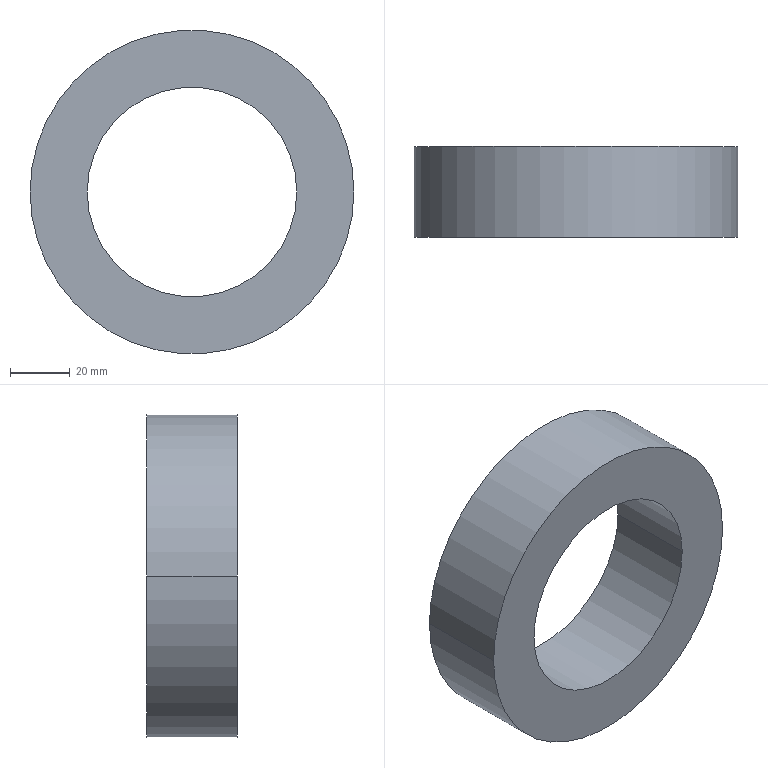Part | STEP file | W468 | 1 solid | 6 faces | box 108.1 x 30.3 x 108.1 mm | volume 161481 mm3 | cylinder 4 | plane 2 | commonest cylinder face diameters 70 x2 108.1 x2
STEP:
#1=CARTESIAN_POINT('',(0.,0.,0.));
#2=DIRECTION('',(0.,0.,1.));
#3=DIRECTION('',(1.,0.,0.));
#4=AXIS2_PLACEMENT_3D('',#1,#2,#3);
#5=CARTESIAN_POINT('',(54.05,0.,0.));
#6=VERTEX_POINT('',#5);
#7=CARTESIAN_POINT('',(-54.05,0.,0.));
#8=VERTEX_POINT('',#7);
#9=CARTESIAN_POINT('',(0.,0.,0.));
#10=DIRECTION('',(0.,-1.,0.));
#11=DIRECTION('',(1.,0.,0.));
#12=AXIS2_PLACEMENT_3D('',#9,#10,#11);
#13=CIRCLE('',#12,54.05);
#14=CARTESIAN_POINT('',(0.,0.,0.));
#15=DIRECTION('',(0.,-1.,0.));
#16=DIRECTION('',(-1.,0.,0.));
#17=AXIS2_PLACEMENT_3D('',#14,#15,#16);
#18=PLANE('',#17);
#19=CARTESIAN_POINT('',(0.,0.));
#20=DIRECTION('',(-1.,0.));
#21=AXIS2_PLACEMENT_2D('',#19,#20);
#22=CIRCLE('',#21,54.05);
#23=(GEOMETRIC_REPRESENTATION_CONTEXT(2)PARAMETRIC_REPRESENTATION_CONTEXT()REPRESENTATION_CONTEXT('',''));
#24=DEFINITIONAL_REPRESENTATION('',(#22),#23);
#25=PCURVE('',#18,#24);
#26=CARTESIAN_POINT('',(0.,31.815,0.));
#27=DIRECTION('',(0.,-1.,0.));
#28=DIRECTION('',(-1.,0.,0.));
#29=AXIS2_PLACEMENT_3D('',#26,#27,#28);
#30=CYLINDRICAL_SURFACE('',#29,54.05);
#31=CARTESIAN_POINT('',(3.142,31.815));
#32=DIRECTION('',(1.,0.));
#33=VECTOR('',#32,1.);
#34=LINE('',#31,#33);
#35=(GEOMETRIC_REPRESENTATION_CONTEXT(2)PARAMETRIC_REPRESENTATION_CONTEXT()REPRESENTATION_CONTEXT('',''));
#36=DEFINITIONAL_REPRESENTATION('',(#34),#35);
#37=PCURVE('',#30,#36);
#38=SURFACE_CURVE('',#13,(#25,#37),.PCURVE_S1.);
#39=EDGE_CURVE('',#6,#8,#38,.T.);
#40=ORIENTED_EDGE('',*,*,#39,.F.);
#41=CARTESIAN_POINT('',(0.,0.,0.));
#42=DIRECTION('',(0.,1.,0.));
#43=DIRECTION('',(1.,0.,0.));
#44=AXIS2_PLACEMENT_3D('',#41,#42,#43);
#45=CIRCLE('',#44,54.05);
#46=CARTESIAN_POINT('',(-54.05,0.));
#47=CARTESIAN_POINT('',(-54.05,93.617));
#48=CARTESIAN_POINT('',(27.025,46.809));
#49=CARTESIAN_POINT('',(108.1,0.));
#50=CARTESIAN_POINT('',(27.025,-46.809));
#51=CARTESIAN_POINT('',(-54.05,-93.617));
#52=CARTESIAN_POINT('',(-54.05,0.));
#53=(BOUNDED_CURVE()B_SPLINE_CURVE(2,(#46,#47,#48,#49,#50,#51,#52),.UNSPECIFIED.,.T.,.F.)B_SPLINE_CURVE_WITH_KNOTS((1,2,2,2,2,1),(-2.094,0.,2.094,4.189,6.283,8.378),.UNSPECIFIED.)CURVE()GEOMETRIC_REPRESENTATION_ITEM()RATIONAL_B_SPLINE_CURVE((1.,0.5,1.,0.5,1.,0.5,1.))REPRESENTATION_ITEM(''));
#54=(GEOMETRIC_REPRESENTATION_CONTEXT(2)PARAMETRIC_REPRESENTATION_CONTEXT()REPRESENTATION_CONTEXT('',''));
#55=DEFINITIONAL_REPRESENTATION('',(#53),#54);
#56=PCURVE('',#18,#55);
#57=CARTESIAN_POINT('',(0.,31.815,0.));
#58=DIRECTION('',(0.,-1.,0.));
#59=DIRECTION('',(-1.,0.,0.));
#60=AXIS2_PLACEMENT_3D('',#57,#58,#59);
#61=CYLINDRICAL_SURFACE('',#60,54.05);
#62=CARTESIAN_POINT('',(3.142,31.815));
#63=DIRECTION('',(-1.,0.));
#64=VECTOR('',#63,1.);
#65=LINE('',#62,#64);
#66=(GEOMETRIC_REPRESENTATION_CONTEXT(2)PARAMETRIC_REPRESENTATION_CONTEXT()REPRESENTATION_CONTEXT('',''));
#67=DEFINITIONAL_REPRESENTATION('',(#65),#66);
#68=PCURVE('',#61,#67);
#69=SURFACE_CURVE('',#45,(#56,#68),.PCURVE_S1.);
#70=EDGE_CURVE('',#6,#8,#69,.T.);
#71=ORIENTED_EDGE('',*,*,#70,.T.);
#72=EDGE_LOOP('',(#40,#71));
#73=FACE_BOUND('',#72,.F.);
#74=CARTESIAN_POINT('',(35.,0.,0.));
#75=VERTEX_POINT('',#74);
#76=CARTESIAN_POINT('',(-35.,0.,0.));
#77=VERTEX_POINT('',#76);
#78=CARTESIAN_POINT('',(0.,0.,0.));
#79=DIRECTION('',(0.,1.,0.));
#80=DIRECTION('',(1.,0.,0.));
#81=AXIS2_PLACEMENT_3D('',#78,#79,#80);
#82=CIRCLE('',#81,35.);
#83=CARTESIAN_POINT('',(-35.,0.));
#84=CARTESIAN_POINT('',(-35.,60.622));
#85=CARTESIAN_POINT('',(17.5,30.311));
#86=CARTESIAN_POINT('',(70.,0.));
#87=CARTESIAN_POINT('',(17.5,-30.311));
#88=CARTESIAN_POINT('',(-35.,-60.622));
#89=CARTESIAN_POINT('',(-35.,0.));
#90=(BOUNDED_CURVE()B_SPLINE_CURVE(2,(#83,#84,#85,#86,#87,#88,#89),.UNSPECIFIED.,.T.,.F.)B_SPLINE_CURVE_WITH_KNOTS((1,2,2,2,2,1),(-2.094,0.,2.094,4.189,6.283,8.378),.UNSPECIFIED.)CURVE()GEOMETRIC_REPRESENTATION_ITEM()RATIONAL_B_SPLINE_CURVE((1.,0.5,1.,0.5,1.,0.5,1.))REPRESENTATION_ITEM(''));
#91=(GEOMETRIC_REPRESENTATION_CONTEXT(2)PARAMETRIC_REPRESENTATION_CONTEXT()REPRESENTATION_CONTEXT('',''));
#92=DEFINITIONAL_REPRESENTATION('',(#90),#91);
#93=PCURVE('',#18,#92);
#94=CARTESIAN_POINT('',(0.,31.815,0.));
#95=DIRECTION('',(0.,-1.,0.));
#96=DIRECTION('',(-1.,0.,0.));
#97=AXIS2_PLACEMENT_3D('',#94,#95,#96);
#98=CYLINDRICAL_SURFACE('',#97,35.);
#99=CARTESIAN_POINT('',(3.142,31.815));
#100=DIRECTION('',(-1.,0.));
#101=VECTOR('',#100,1.);
#102=LINE('',#99,#101);
#103=(GEOMETRIC_REPRESENTATION_CONTEXT(2)PARAMETRIC_REPRESENTATION_CONTEXT()REPRESENTATION_CONTEXT('',''));
#104=DEFINITIONAL_REPRESENTATION('',(#102),#103);
#105=PCURVE('',#98,#104);
#106=SURFACE_CURVE('',#82,(#93,#105),.PCURVE_S1.);
#107=EDGE_CURVE('',#75,#77,#106,.T.);
#108=ORIENTED_EDGE('',*,*,#107,.F.);
#109=CARTESIAN_POINT('',(0.,0.,0.));
#110=DIRECTION('',(0.,-1.,0.));
#111=DIRECTION('',(1.,0.,0.));
#112=AXIS2_PLACEMENT_3D('',#109,#110,#111);
#113=CIRCLE('',#112,35.);
#114=CARTESIAN_POINT('',(0.,0.));
#115=DIRECTION('',(-1.,0.));
#116=AXIS2_PLACEMENT_2D('',#114,#115);
#117=CIRCLE('',#116,35.);
#118=(GEOMETRIC_REPRESENTATION_CONTEXT(2)PARAMETRIC_REPRESENTATION_CONTEXT()REPRESENTATION_CONTEXT('',''));
#119=DEFINITIONAL_REPRESENTATION('',(#117),#118);
#120=PCURVE('',#18,#119);
#121=CARTESIAN_POINT('',(0.,31.815,0.));
#122=DIRECTION('',(0.,-1.,0.));
#123=DIRECTION('',(-1.,0.,0.));
#124=AXIS2_PLACEMENT_3D('',#121,#122,#123);
#125=CYLINDRICAL_SURFACE('',#124,35.);
#126=CARTESIAN_POINT('',(3.142,31.815));
#127=DIRECTION('',(1.,0.));
#128=VECTOR('',#127,1.);
#129=LINE('',#126,#128);
#130=(GEOMETRIC_REPRESENTATION_CONTEXT(2)PARAMETRIC_REPRESENTATION_CONTEXT()REPRESENTATION_CONTEXT('',''));
#131=DEFINITIONAL_REPRESENTATION('',(#129),#130);
#132=PCURVE('',#125,#131);
#133=SURFACE_CURVE('',#113,(#120,#132),.PCURVE_S1.);
#134=EDGE_CURVE('',#75,#77,#133,.T.);
#135=ORIENTED_EDGE('',*,*,#134,.T.);
#136=EDGE_LOOP('',(#108,#135));
#137=FACE_BOUND('',#136,.F.);
#138=ADVANCED_FACE('',(#73,#137),#18,.T.);
#139=CARTESIAN_POINT('',(54.05,30.3,0.));
#140=VERTEX_POINT('',#139);
#141=CARTESIAN_POINT('',(-54.05,30.3,0.));
#142=VERTEX_POINT('',#141);
#143=CARTESIAN_POINT('',(0.,30.3,0.));
#144=DIRECTION('',(0.,-1.,0.));
#145=DIRECTION('',(1.,0.,0.));
#146=AXIS2_PLACEMENT_3D('',#143,#144,#145);
#147=CIRCLE('',#146,54.05);
#148=CARTESIAN_POINT('',(3.142,1.515));
#149=DIRECTION('',(1.,0.));
#150=VECTOR('',#149,1.);
#151=LINE('',#148,#150);
#152=(GEOMETRIC_REPRESENTATION_CONTEXT(2)PARAMETRIC_REPRESENTATION_CONTEXT()REPRESENTATION_CONTEXT('',''));
#153=DEFINITIONAL_REPRESENTATION('',(#151),#152);
#154=PCURVE('',#30,#153);
#155=CARTESIAN_POINT('',(0.,30.3,0.));
#156=DIRECTION('',(0.,-1.,0.));
#157=DIRECTION('',(-1.,0.,0.));
#158=AXIS2_PLACEMENT_3D('',#155,#156,#157);
#159=PLANE('',#158);
#160=CARTESIAN_POINT('',(0.,0.));
#161=DIRECTION('',(-1.,0.));
#162=AXIS2_PLACEMENT_2D('',#160,#161);
#163=CIRCLE('',#162,54.05);
#164=(GEOMETRIC_REPRESENTATION_CONTEXT(2)PARAMETRIC_REPRESENTATION_CONTEXT()REPRESENTATION_CONTEXT('',''));
#165=DEFINITIONAL_REPRESENTATION('',(#163),#164);
#166=PCURVE('',#159,#165);
#167=SURFACE_CURVE('',#147,(#154,#166),.PCURVE_S1.);
#168=EDGE_CURVE('',#140,#142,#167,.T.);
#169=ORIENTED_EDGE('',*,*,#168,.T.);
#170=CARTESIAN_POINT('',(-54.05,0.,0.));
#171=DIRECTION('',(0.,1.,0.));
#172=VECTOR('',#171,1.);
#173=LINE('',#170,#172);
#174=CARTESIAN_POINT('',(6.283,31.815));
#175=DIRECTION('',(0.,-1.));
#176=VECTOR('',#175,1.);
#177=LINE('',#174,#176);
#178=(GEOMETRIC_REPRESENTATION_CONTEXT(2)PARAMETRIC_REPRESENTATION_CONTEXT()REPRESENTATION_CONTEXT('',''));
#179=DEFINITIONAL_REPRESENTATION('',(#177),#178);
#180=PCURVE('',#30,#179);
#181=CARTESIAN_POINT('',(0.,31.815));
#182=DIRECTION('',(0.,-1.));
#183=VECTOR('',#182,1.);
#184=LINE('',#181,#183);
#185=(GEOMETRIC_REPRESENTATION_CONTEXT(2)PARAMETRIC_REPRESENTATION_CONTEXT()REPRESENTATION_CONTEXT('',''));
#186=DEFINITIONAL_REPRESENTATION('',(#184),#185);
#187=PCURVE('',#61,#186);
#188=SURFACE_CURVE('',#173,(#180,#187),.PCURVE_S1.);
#189=EDGE_CURVE('',#8,#142,#188,.T.);
#190=ORIENTED_EDGE('',*,*,#189,.F.);
#191=ORIENTED_EDGE('',*,*,#39,.F.);
#192=CARTESIAN_POINT('',(54.05,0.,0.));
#193=DIRECTION('',(0.,1.,0.));
#194=VECTOR('',#193,1.);
#195=LINE('',#192,#194);
#196=CARTESIAN_POINT('',(3.142,31.815));
#197=DIRECTION('',(0.,-1.));
#198=VECTOR('',#197,1.);
#199=LINE('',#196,#198);
#200=(GEOMETRIC_REPRESENTATION_CONTEXT(2)PARAMETRIC_REPRESENTATION_CONTEXT()REPRESENTATION_CONTEXT('',''));
#201=DEFINITIONAL_REPRESENTATION('',(#199),#200);
#202=PCURVE('',#30,#201);
#203=CARTESIAN_POINT('',(3.142,31.815));
#204=DIRECTION('',(0.,-1.));
#205=VECTOR('',#204,1.);
#206=LINE('',#203,#205);
#207=(GEOMETRIC_REPRESENTATION_CONTEXT(2)PARAMETRIC_REPRESENTATION_CONTEXT()REPRESENTATION_CONTEXT('',''));
#208=DEFINITIONAL_REPRESENTATION('',(#206),#207);
#209=PCURVE('',#61,#208);
#210=SURFACE_CURVE('',#195,(#202,#209),.PCURVE_S1.);
#211=EDGE_CURVE('',#6,#140,#210,.T.);
#212=ORIENTED_EDGE('',*,*,#211,.T.);
#213=EDGE_LOOP('',(#169,#190,#191,#212));
#214=FACE_BOUND('',#213,.T.);
#215=ADVANCED_FACE('',(#214),#30,.T.);
#216=ORIENTED_EDGE('',*,*,#70,.T.);
#217=ORIENTED_EDGE('',*,*,#189,.T.);
#218=CARTESIAN_POINT('',(0.,30.3,0.));
#219=DIRECTION('',(0.,1.,0.));
#220=DIRECTION('',(1.,0.,0.));
#221=AXIS2_PLACEMENT_3D('',#218,#219,#220);
#222=CIRCLE('',#221,54.05);
#223=CARTESIAN_POINT('',(3.142,1.515));
#224=DIRECTION('',(-1.,0.));
#225=VECTOR('',#224,1.);
#226=LINE('',#223,#225);
#227=(GEOMETRIC_REPRESENTATION_CONTEXT(2)PARAMETRIC_REPRESENTATION_CONTEXT()REPRESENTATION_CONTEXT('',''));
#228=DEFINITIONAL_REPRESENTATION('',(#226),#227);
#229=PCURVE('',#61,#228);
#230=CARTESIAN_POINT('',(-54.05,0.));
#231=CARTESIAN_POINT('',(-54.05,93.617));
#232=CARTESIAN_POINT('',(27.025,46.809));
#233=CARTESIAN_POINT('',(108.1,0.));
#234=CARTESIAN_POINT('',(27.025,-46.809));
#235=CARTESIAN_POINT('',(-54.05,-93.617));
#236=CARTESIAN_POINT('',(-54.05,0.));
#237=(BOUNDED_CURVE()B_SPLINE_CURVE(2,(#230,#231,#232,#233,#234,#235,#236),.UNSPECIFIED.,.T.,.F.)B_SPLINE_CURVE_WITH_KNOTS((1,2,2,2,2,1),(-2.094,0.,2.094,4.189,6.283,8.378),.UNSPECIFIED.)CURVE()GEOMETRIC_REPRESENTATION_ITEM()RATIONAL_B_SPLINE_CURVE((1.,0.5,1.,0.5,1.,0.5,1.))REPRESENTATION_ITEM(''));
#238=(GEOMETRIC_REPRESENTATION_CONTEXT(2)PARAMETRIC_REPRESENTATION_CONTEXT()REPRESENTATION_CONTEXT('',''));
#239=DEFINITIONAL_REPRESENTATION('',(#237),#238);
#240=PCURVE('',#159,#239);
#241=SURFACE_CURVE('',#222,(#229,#240),.PCURVE_S1.);
#242=EDGE_CURVE('',#140,#142,#241,.T.);
#243=ORIENTED_EDGE('',*,*,#242,.F.);
#244=ORIENTED_EDGE('',*,*,#211,.F.);
#245=EDGE_LOOP('',(#216,#217,#243,#244));
#246=FACE_BOUND('',#245,.T.);
#247=ADVANCED_FACE('',(#246),#61,.T.);
#248=ORIENTED_EDGE('',*,*,#242,.F.);
#249=ORIENTED_EDGE('',*,*,#168,.T.);
#250=EDGE_LOOP('',(#248,#249));
#251=FACE_BOUND('',#250,.F.);
#252=CARTESIAN_POINT('',(35.,30.3,0.));
#253=VERTEX_POINT('',#252);
#254=CARTESIAN_POINT('',(-35.,30.3,0.));
#255=VERTEX_POINT('',#254);
#256=CARTESIAN_POINT('',(0.,30.3,0.));
#257=DIRECTION('',(0.,-1.,0.));
#258=DIRECTION('',(1.,0.,0.));
#259=AXIS2_PLACEMENT_3D('',#256,#257,#258);
#260=CIRCLE('',#259,35.);
#261=CARTESIAN_POINT('',(0.,0.));
#262=DIRECTION('',(-1.,0.));
#263=AXIS2_PLACEMENT_2D('',#261,#262);
#264=CIRCLE('',#263,35.);
#265=(GEOMETRIC_REPRESENTATION_CONTEXT(2)PARAMETRIC_REPRESENTATION_CONTEXT()REPRESENTATION_CONTEXT('',''));
#266=DEFINITIONAL_REPRESENTATION('',(#264),#265);
#267=PCURVE('',#159,#266);
#268=CARTESIAN_POINT('',(3.142,1.515));
#269=DIRECTION('',(1.,0.));
#270=VECTOR('',#269,1.);
#271=LINE('',#268,#270);
#272=(GEOMETRIC_REPRESENTATION_CONTEXT(2)PARAMETRIC_REPRESENTATION_CONTEXT()REPRESENTATION_CONTEXT('',''));
#273=DEFINITIONAL_REPRESENTATION('',(#271),#272);
#274=PCURVE('',#125,#273);
#275=SURFACE_CURVE('',#260,(#267,#274),.PCURVE_S1.);
#276=EDGE_CURVE('',#253,#255,#275,.T.);
#277=ORIENTED_EDGE('',*,*,#276,.F.);
#278=CARTESIAN_POINT('',(0.,30.3,0.));
#279=DIRECTION('',(0.,1.,0.));
#280=DIRECTION('',(1.,0.,0.));
#281=AXIS2_PLACEMENT_3D('',#278,#279,#280);
#282=CIRCLE('',#281,35.);
#283=CARTESIAN_POINT('',(-35.,0.));
#284=CARTESIAN_POINT('',(-35.,60.622));
#285=CARTESIAN_POINT('',(17.5,30.311));
#286=CARTESIAN_POINT('',(70.,0.));
#287=CARTESIAN_POINT('',(17.5,-30.311));
#288=CARTESIAN_POINT('',(-35.,-60.622));
#289=CARTESIAN_POINT('',(-35.,0.));
#290=(BOUNDED_CURVE()B_SPLINE_CURVE(2,(#283,#284,#285,#286,#287,#288,#289),.UNSPECIFIED.,.T.,.F.)B_SPLINE_CURVE_WITH_KNOTS((1,2,2,2,2,1),(-2.094,0.,2.094,4.189,6.283,8.378),.UNSPECIFIED.)CURVE()GEOMETRIC_REPRESENTATION_ITEM()RATIONAL_B_SPLINE_CURVE((1.,0.5,1.,0.5,1.,0.5,1.))REPRESENTATION_ITEM(''));
#291=(GEOMETRIC_REPRESENTATION_CONTEXT(2)PARAMETRIC_REPRESENTATION_CONTEXT()REPRESENTATION_CONTEXT('',''));
#292=DEFINITIONAL_REPRESENTATION('',(#290),#291);
#293=PCURVE('',#159,#292);
#294=CARTESIAN_POINT('',(3.142,1.515));
#295=DIRECTION('',(-1.,0.));
#296=VECTOR('',#295,1.);
#297=LINE('',#294,#296);
#298=(GEOMETRIC_REPRESENTATION_CONTEXT(2)PARAMETRIC_REPRESENTATION_CONTEXT()REPRESENTATION_CONTEXT('',''));
#299=DEFINITIONAL_REPRESENTATION('',(#297),#298);
#300=PCURVE('',#98,#299);
#301=SURFACE_CURVE('',#282,(#293,#300),.PCURVE_S1.);
#302=EDGE_CURVE('',#253,#255,#301,.T.);
#303=ORIENTED_EDGE('',*,*,#302,.T.);
#304=EDGE_LOOP('',(#277,#303));
#305=FACE_BOUND('',#304,.F.);
#306=ADVANCED_FACE('',(#251,#305),#159,.F.);
#307=CARTESIAN_POINT('',(35.,30.3,0.));
#308=DIRECTION('',(0.,-1.,0.));
#309=VECTOR('',#308,1.);
#310=LINE('',#307,#309);
#311=CARTESIAN_POINT('',(3.142,1.515));
#312=DIRECTION('',(0.,1.));
#313=VECTOR('',#312,1.);
#314=LINE('',#311,#313);
#315=(GEOMETRIC_REPRESENTATION_CONTEXT(2)PARAMETRIC_REPRESENTATION_CONTEXT()REPRESENTATION_CONTEXT('',''));
#316=DEFINITIONAL_REPRESENTATION('',(#314),#315);
#317=PCURVE('',#125,#316);
#318=CARTESIAN_POINT('',(3.142,1.515));
#319=DIRECTION('',(0.,1.));
#320=VECTOR('',#319,1.);
#321=LINE('',#318,#320);
#322=(GEOMETRIC_REPRESENTATION_CONTEXT(2)PARAMETRIC_REPRESENTATION_CONTEXT()REPRESENTATION_CONTEXT('',''));
#323=DEFINITIONAL_REPRESENTATION('',(#321),#322);
#324=PCURVE('',#98,#323);
#325=SURFACE_CURVE('',#310,(#317,#324),.PCURVE_S1.);
#326=EDGE_CURVE('',#253,#75,#325,.T.);
#327=ORIENTED_EDGE('',*,*,#326,.F.);
#328=ORIENTED_EDGE('',*,*,#276,.T.);
#329=CARTESIAN_POINT('',(-35.,30.3,0.));
#330=DIRECTION('',(0.,-1.,0.));
#331=VECTOR('',#330,1.);
#332=LINE('',#329,#331);
#333=CARTESIAN_POINT('',(6.283,1.515));
#334=DIRECTION('',(0.,1.));
#335=VECTOR('',#334,1.);
#336=LINE('',#333,#335);
#337=(GEOMETRIC_REPRESENTATION_CONTEXT(2)PARAMETRIC_REPRESENTATION_CONTEXT()REPRESENTATION_CONTEXT('',''));
#338=DEFINITIONAL_REPRESENTATION('',(#336),#337);
#339=PCURVE('',#125,#338);
#340=CARTESIAN_POINT('',(0.,1.515));
#341=DIRECTION('',(0.,1.));
#342=VECTOR('',#341,1.);
#343=LINE('',#340,#342);
#344=(GEOMETRIC_REPRESENTATION_CONTEXT(2)PARAMETRIC_REPRESENTATION_CONTEXT()REPRESENTATION_CONTEXT('',''));
#345=DEFINITIONAL_REPRESENTATION('',(#343),#344);
#346=PCURVE('',#98,#345);
#347=SURFACE_CURVE('',#332,(#339,#346),.PCURVE_S1.);
#348=EDGE_CURVE('',#255,#77,#347,.T.);
#349=ORIENTED_EDGE('',*,*,#348,.T.);
#350=ORIENTED_EDGE('',*,*,#134,.F.);
#351=EDGE_LOOP('',(#327,#328,#349,#350));
#352=FACE_BOUND('',#351,.F.);
#353=ADVANCED_FACE('',(#352),#125,.F.);
#354=ORIENTED_EDGE('',*,*,#326,.T.);
#355=ORIENTED_EDGE('',*,*,#107,.T.);
#356=ORIENTED_EDGE('',*,*,#348,.F.);
#357=ORIENTED_EDGE('',*,*,#302,.F.);
#358=EDGE_LOOP('',(#354,#355,#356,#357));
#359=FACE_BOUND('',#358,.F.);
#360=ADVANCED_FACE('',(#359),#98,.F.);
#361=CLOSED_SHELL('',(#138,#215,#247,#306,#353,#360));
#362=MANIFOLD_SOLID_BREP('',#361);
#363=(LENGTH_UNIT()NAMED_UNIT(*)SI_UNIT(.MILLI.,.METRE.));
#364=UNCERTAINTY_MEASURE_WITH_UNIT(LENGTH_MEASURE(0.0000001),#363,'','');
#365=(NAMED_UNIT(*)PLANE_ANGLE_UNIT()SI_UNIT($,.RADIAN.));
#366=(NAMED_UNIT(*)SI_UNIT($,.STERADIAN.)SOLID_ANGLE_UNIT());
#367=(GEOMETRIC_REPRESENTATION_CONTEXT(3)GLOBAL_UNCERTAINTY_ASSIGNED_CONTEXT((#364))GLOBAL_UNIT_ASSIGNED_CONTEXT((#363,#365,#366))REPRESENTATION_CONTEXT('',''));
#368=ADVANCED_BREP_SHAPE_REPRESENTATION('',(#4,#362),#367);